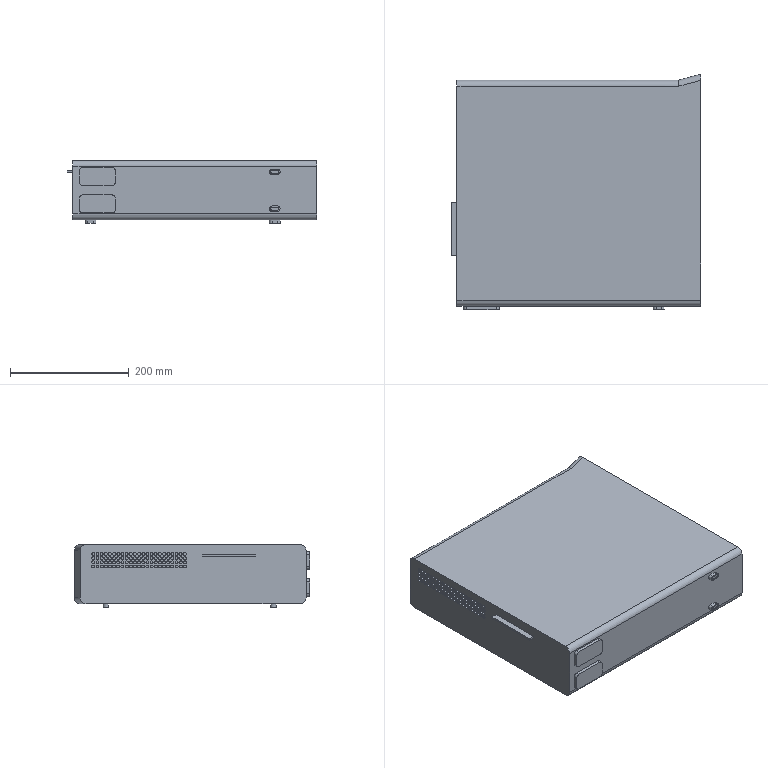Part | STEP file | Guide wheel mechanism revised.sldasm-Part-192 | 1 solid | 1633 faces | box 420.5 x 396 x 106 mm | volume 15546252 mm3 | plane 901 | cylinder 714 | spline 16 | cone 2 | commonest cylinder face diameters 2 x468 5 x200 9 x16 10 x8 20 x6 3 x4